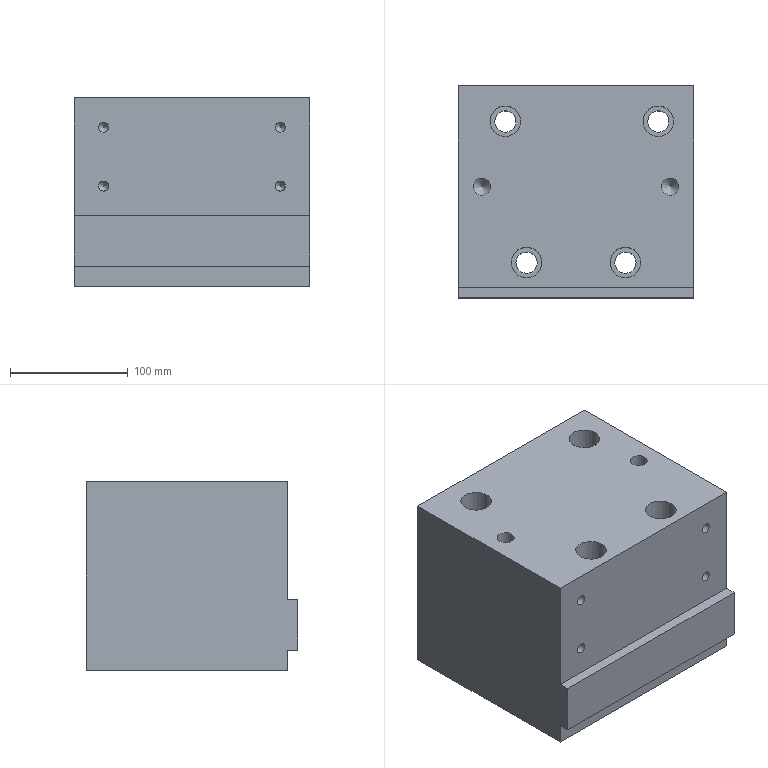Part | STEP file | lll_id3798_x_t | 1 solid | 34 faces | box 200 x 180 x 160 mm | volume 5233712 mm3 | plane 14 | cylinder 14 | cone 6 | commonest cylinder face diameters 8.506 x4 18.009 x4 26.008 x4 14.506 x2
STEP:
#1=CARTESIAN_POINT('',(1890.,537.377,65.));
#2=VERTEX_POINT('',#1);
#3=CARTESIAN_POINT('',(1890.,366.377,65.));
#4=VERTEX_POINT('',#3);
#5=CARTESIAN_POINT('',(1890.,293.877,65.));
#6=DIRECTION('',(0.,-1.,0.));
#7=VECTOR('',#6,1.);
#8=LINE('',#5,#7);
#9=EDGE_CURVE('',#2,#4,#8,.T.);
#10=ORIENTED_EDGE('',*,*,#9,.F.);
#11=CARTESIAN_POINT('',(1690.,537.377,65.));
#12=VERTEX_POINT('',#11);
#13=CARTESIAN_POINT('',(1665.,537.377,65.));
#14=DIRECTION('',(1.,0.,0.));
#15=VECTOR('',#14,1.);
#16=LINE('',#13,#15);
#17=EDGE_CURVE('',#12,#2,#16,.T.);
#18=ORIENTED_EDGE('',*,*,#17,.F.);
#19=CARTESIAN_POINT('',(1690.,366.377,65.));
#20=VERTEX_POINT('',#19);
#21=CARTESIAN_POINT('',(1690.,293.877,65.));
#22=DIRECTION('',(0.,1.,0.));
#23=VECTOR('',#22,1.);
#24=LINE('',#21,#23);
#25=EDGE_CURVE('',#20,#12,#24,.T.);
#26=ORIENTED_EDGE('',*,*,#25,.F.);
#27=CARTESIAN_POINT('',(1665.,366.377,65.));
#28=DIRECTION('',(-1.,0.,0.));
#29=VECTOR('',#28,1.);
#30=LINE('',#27,#29);
#31=EDGE_CURVE('',#4,#20,#30,.T.);
#32=ORIENTED_EDGE('',*,*,#31,.F.);
#33=EDGE_LOOP('',(#10,#18,#26,#32));
#34=FACE_BOUND('',#33,.T.);
#35=CARTESIAN_POINT('',(1873.004,507.377,65.));
#36=VERTEX_POINT('',#35);
#37=CARTESIAN_POINT('',(1860.,507.377,65.));
#38=DIRECTION('',(0.,0.,-1.));
#39=DIRECTION('',(1.,0.,0.));
#40=AXIS2_PLACEMENT_3D('',#37,#38,#39);
#41=CIRCLE('',#40,13.004);
#42=EDGE_CURVE('',#36,#36,#41,.T.);
#43=ORIENTED_EDGE('',*,*,#42,.T.);
#44=EDGE_LOOP('',(#43));
#45=FACE_BOUND('',#44,.T.);
#46=CARTESIAN_POINT('',(1845.004,387.377,65.));
#47=VERTEX_POINT('',#46);
#48=CARTESIAN_POINT('',(1832.,387.377,65.));
#49=DIRECTION('',(0.,0.,-1.));
#50=DIRECTION('',(1.,0.,0.));
#51=AXIS2_PLACEMENT_3D('',#48,#49,#50);
#52=CIRCLE('',#51,13.004);
#53=EDGE_CURVE('',#47,#47,#52,.T.);
#54=ORIENTED_EDGE('',*,*,#53,.T.);
#55=EDGE_LOOP('',(#54));
#56=FACE_BOUND('',#55,.T.);
#57=CARTESIAN_POINT('',(1877.253,451.877,65.));
#58=VERTEX_POINT('',#57);
#59=CARTESIAN_POINT('',(1870.,451.877,65.));
#60=DIRECTION('',(0.,0.,-1.));
#61=DIRECTION('',(1.,0.,0.));
#62=AXIS2_PLACEMENT_3D('',#59,#60,#61);
#63=CIRCLE('',#62,7.253);
#64=EDGE_CURVE('',#58,#58,#63,.T.);
#65=ORIENTED_EDGE('',*,*,#64,.T.);
#66=EDGE_LOOP('',(#65));
#67=FACE_BOUND('',#66,.T.);
#68=CARTESIAN_POINT('',(1702.747,451.877,65.));
#69=VERTEX_POINT('',#68);
#70=CARTESIAN_POINT('',(1710.,451.877,65.));
#71=DIRECTION('',(0.,0.,1.));
#72=DIRECTION('',(-1.,0.,0.));
#73=AXIS2_PLACEMENT_3D('',#70,#71,#72);
#74=CIRCLE('',#73,7.253);
#75=EDGE_CURVE('',#69,#69,#74,.T.);
#76=ORIENTED_EDGE('',*,*,#75,.F.);
#77=EDGE_LOOP('',(#76));
#78=FACE_BOUND('',#77,.T.);
#79=CARTESIAN_POINT('',(1734.996,387.377,65.));
#80=VERTEX_POINT('',#79);
#81=CARTESIAN_POINT('',(1748.,387.377,65.));
#82=DIRECTION('',(0.,0.,-1.));
#83=DIRECTION('',(-1.,0.,0.));
#84=AXIS2_PLACEMENT_3D('',#81,#82,#83);
#85=CIRCLE('',#84,13.004);
#86=EDGE_CURVE('',#80,#80,#85,.T.);
#87=ORIENTED_EDGE('',*,*,#86,.T.);
#88=EDGE_LOOP('',(#87));
#89=FACE_BOUND('',#88,.T.);
#90=CARTESIAN_POINT('',(1716.996,507.377,65.));
#91=VERTEX_POINT('',#90);
#92=CARTESIAN_POINT('',(1730.,507.377,65.));
#93=DIRECTION('',(0.,0.,-1.));
#94=DIRECTION('',(-1.,0.,0.));
#95=AXIS2_PLACEMENT_3D('',#92,#93,#94);
#96=CIRCLE('',#95,13.004);
#97=EDGE_CURVE('',#91,#91,#96,.T.);
#98=ORIENTED_EDGE('',*,*,#97,.T.);
#99=EDGE_LOOP('',(#98));
#100=FACE_BOUND('',#99,.T.);
#101=CARTESIAN_POINT('',(1665.,293.877,65.));
#102=DIRECTION('',(0.,0.,1.));
#103=DIRECTION('',(-1.,0.,0.));
#104=AXIS2_PLACEMENT_3D('',#101,#102,#103);
#105=PLANE('',#104);
#106=ADVANCED_FACE('',(#34,#45,#56,#67,#78,#89,#100),#105,.T.);
#107=CARTESIAN_POINT('',(1890.,537.377,-95.));
#108=VERTEX_POINT('',#107);
#109=CARTESIAN_POINT('',(1890.,537.377,-120.));
#110=DIRECTION('',(0.,0.,1.));
#111=VECTOR('',#110,1.);
#112=LINE('',#109,#111);
#113=EDGE_CURVE('',#108,#2,#112,.T.);
#114=ORIENTED_EDGE('',*,*,#113,.F.);
#115=CARTESIAN_POINT('',(1690.,537.377,-95.));
#116=VERTEX_POINT('',#115);
#117=CARTESIAN_POINT('',(1665.,537.377,-95.));
#118=DIRECTION('',(1.,0.,0.));
#119=VECTOR('',#118,1.);
#120=LINE('',#117,#119);
#121=EDGE_CURVE('',#116,#108,#120,.T.);
#122=ORIENTED_EDGE('',*,*,#121,.F.);
#123=CARTESIAN_POINT('',(1690.,537.377,-105.));
#124=DIRECTION('',(0.,0.,1.));
#125=VECTOR('',#124,1.);
#126=LINE('',#123,#125);
#127=EDGE_CURVE('',#116,#12,#126,.T.);
#128=ORIENTED_EDGE('',*,*,#127,.T.);
#129=ORIENTED_EDGE('',*,*,#17,.T.);
#130=EDGE_LOOP('',(#114,#122,#128,#129));
#131=FACE_OUTER_BOUND('',#130,.T.);
#132=CARTESIAN_POINT('',(1665.,537.377,-120.));
#133=DIRECTION('',(0.,1.,0.));
#134=DIRECTION('',(0.,0.,-1.));
#135=AXIS2_PLACEMENT_3D('',#132,#133,#134);
#136=PLANE('',#135);
#137=ADVANCED_FACE('',(#131),#136,.T.);
#138=CARTESIAN_POINT('',(1841.005,387.377,-55.));
#139=VERTEX_POINT('',#138);
#140=CARTESIAN_POINT('',(1832.,387.377,-55.));
#141=DIRECTION('',(0.,0.,-1.));
#142=DIRECTION('',(1.,0.,0.));
#143=AXIS2_PLACEMENT_3D('',#140,#141,#142);
#144=CIRCLE('',#143,9.005);
#145=EDGE_CURVE('',#139,#139,#144,.T.);
#146=ORIENTED_EDGE('',*,*,#145,.T.);
#147=EDGE_LOOP('',(#146));
#148=FACE_BOUND('',#147,.T.);
#149=CARTESIAN_POINT('',(1845.004,387.377,-55.));
#150=VERTEX_POINT('',#149);
#151=CARTESIAN_POINT('',(1832.,387.377,-55.));
#152=DIRECTION('',(0.,0.,-1.));
#153=DIRECTION('',(1.,0.,0.));
#154=AXIS2_PLACEMENT_3D('',#151,#152,#153);
#155=CIRCLE('',#154,13.004);
#156=EDGE_CURVE('',#150,#150,#155,.T.);
#157=ORIENTED_EDGE('',*,*,#156,.F.);
#158=EDGE_LOOP('',(#157));
#159=FACE_BOUND('',#158,.T.);
#160=CARTESIAN_POINT('',(1832.,387.377,-55.));
#161=DIRECTION('',(0.,0.,-1.));
#162=DIRECTION('',(-1.,0.,0.));
#163=AXIS2_PLACEMENT_3D('',#160,#161,#162);
#164=PLANE('',#163);
#165=ADVANCED_FACE('',(#148,#159),#164,.F.);
#166=ORIENTED_EDGE('',*,*,#145,.F.);
#167=EDGE_LOOP('',(#166));
#168=FACE_BOUND('',#167,.T.);
#169=CARTESIAN_POINT('',(1841.005,387.377,-95.));
#170=VERTEX_POINT('',#169);
#171=CARTESIAN_POINT('',(1832.,387.377,-95.));
#172=DIRECTION('',(0.,0.,-1.));
#173=DIRECTION('',(1.,0.,0.));
#174=AXIS2_PLACEMENT_3D('',#171,#172,#173);
#175=CIRCLE('',#174,9.005);
#176=EDGE_CURVE('',#170,#170,#175,.T.);
#177=ORIENTED_EDGE('',*,*,#176,.T.);
#178=EDGE_LOOP('',(#177));
#179=FACE_BOUND('',#178,.T.);
#180=CARTESIAN_POINT('',(1832.,387.377,67.));
#181=DIRECTION('',(0.,0.,-1.));
#182=DIRECTION('',(1.,0.,0.));
#183=AXIS2_PLACEMENT_3D('',#180,#181,#182);
#184=CYLINDRICAL_SURFACE('',#183,9.005);
#185=ADVANCED_FACE('',(#168,#179),#184,.F.);
#186=ORIENTED_EDGE('',*,*,#156,.T.);
#187=EDGE_LOOP('',(#186));
#188=FACE_BOUND('',#187,.T.);
#189=ORIENTED_EDGE('',*,*,#53,.F.);
#190=EDGE_LOOP('',(#189));
#191=FACE_BOUND('',#190,.T.);
#192=CARTESIAN_POINT('',(1832.,387.377,65.));
#193=DIRECTION('',(0.,0.,-1.));
#194=DIRECTION('',(1.,0.,0.));
#195=AXIS2_PLACEMENT_3D('',#192,#193,#194);
#196=CYLINDRICAL_SURFACE('',#195,13.004);
#197=ADVANCED_FACE('',(#188,#191),#196,.F.);
#198=CARTESIAN_POINT('',(1715.,401.383,40.));
#199=VERTEX_POINT('',#198);
#200=VERTEX_LOOP('',#199);
#201=FACE_BOUND('',#200,.T.);
#202=CARTESIAN_POINT('',(1715.,397.13,35.747));
#203=VERTEX_POINT('',#202);
#204=CARTESIAN_POINT('',(1715.,397.13,40.));
#205=DIRECTION('',(0.,1.,0.));
#206=DIRECTION('',(0.,0.,-1.));
#207=AXIS2_PLACEMENT_3D('',#204,#205,#206);
#208=CIRCLE('',#207,4.253);
#209=EDGE_CURVE('',#203,#203,#208,.T.);
#210=ORIENTED_EDGE('',*,*,#209,.F.);
#211=EDGE_LOOP('',(#210));
#212=FACE_BOUND('',#211,.T.);
#213=CARTESIAN_POINT('',(1715.,397.13,40.));
#214=DIRECTION('',(0.,-1.,0.));
#215=DIRECTION('',(0.,0.,1.));
#216=AXIS2_PLACEMENT_3D('',#213,#214,#215);
#217=CONICAL_SURFACE('',#216,4.253,45.);
#218=ADVANCED_FACE('',(#201,#212),#217,.F.);
#219=CARTESIAN_POINT('',(1865.,401.383,40.));
#220=VERTEX_POINT('',#219);
#221=VERTEX_LOOP('',#220);
#222=FACE_BOUND('',#221,.T.);
#223=CARTESIAN_POINT('',(1865.,397.13,35.747));
#224=VERTEX_POINT('',#223);
#225=CARTESIAN_POINT('',(1865.,397.13,40.));
#226=DIRECTION('',(0.,1.,0.));
#227=DIRECTION('',(0.,0.,-1.));
#228=AXIS2_PLACEMENT_3D('',#225,#226,#227);
#229=CIRCLE('',#228,4.253);
#230=EDGE_CURVE('',#224,#224,#229,.T.);
#231=ORIENTED_EDGE('',*,*,#230,.F.);
#232=EDGE_LOOP('',(#231));
#233=FACE_BOUND('',#232,.T.);
#234=CARTESIAN_POINT('',(1865.,397.13,40.));
#235=DIRECTION('',(0.,-1.,0.));
#236=DIRECTION('',(0.,0.,1.));
#237=AXIS2_PLACEMENT_3D('',#234,#235,#236);
#238=CONICAL_SURFACE('',#237,4.253,45.);
#239=ADVANCED_FACE('',(#222,#233),#238,.F.);
#240=CARTESIAN_POINT('',(1715.,401.383,-10.));
#241=VERTEX_POINT('',#240);
#242=VERTEX_LOOP('',#241);
#243=FACE_BOUND('',#242,.T.);
#244=CARTESIAN_POINT('',(1715.,397.13,-14.253));
#245=VERTEX_POINT('',#244);
#246=CARTESIAN_POINT('',(1715.,397.13,-10.));
#247=DIRECTION('',(0.,1.,0.));
#248=DIRECTION('',(0.,0.,-1.));
#249=AXIS2_PLACEMENT_3D('',#246,#247,#248);
#250=CIRCLE('',#249,4.253);
#251=EDGE_CURVE('',#245,#245,#250,.T.);
#252=ORIENTED_EDGE('',*,*,#251,.F.);
#253=EDGE_LOOP('',(#252));
#254=FACE_BOUND('',#253,.T.);
#255=CARTESIAN_POINT('',(1715.,397.13,-10.));
#256=DIRECTION('',(0.,-1.,0.));
#257=DIRECTION('',(0.,0.,1.));
#258=AXIS2_PLACEMENT_3D('',#255,#256,#257);
#259=CONICAL_SURFACE('',#258,4.253,45.);
#260=ADVANCED_FACE('',(#243,#254),#259,.F.);
#261=CARTESIAN_POINT('',(1865.,401.383,-10.));
#262=VERTEX_POINT('',#261);
#263=VERTEX_LOOP('',#262);
#264=FACE_BOUND('',#263,.T.);
#265=CARTESIAN_POINT('',(1865.,397.13,-14.253));
#266=VERTEX_POINT('',#265);
#267=CARTESIAN_POINT('',(1865.,397.13,-10.));
#268=DIRECTION('',(0.,1.,0.));
#269=DIRECTION('',(0.,0.,-1.));
#270=AXIS2_PLACEMENT_3D('',#267,#268,#269);
#271=CIRCLE('',#270,4.253);
#272=EDGE_CURVE('',#266,#266,#271,.T.);
#273=ORIENTED_EDGE('',*,*,#272,.F.);
#274=EDGE_LOOP('',(#273));
#275=FACE_BOUND('',#274,.T.);
#276=CARTESIAN_POINT('',(1865.,397.13,-10.));
#277=DIRECTION('',(0.,-1.,0.));
#278=DIRECTION('',(0.,0.,1.));
#279=AXIS2_PLACEMENT_3D('',#276,#277,#278);
#280=CONICAL_SURFACE('',#279,4.253,45.);
#281=ADVANCED_FACE('',(#264,#275),#280,.F.);
#282=CARTESIAN_POINT('',(1710.,451.877,21.994));
#283=VERTEX_POINT('',#282);
#284=VERTEX_LOOP('',#283);
#285=FACE_BOUND('',#284,.T.);
#286=CARTESIAN_POINT('',(1717.253,451.877,29.247));
#287=VERTEX_POINT('',#286);
#288=CARTESIAN_POINT('',(1710.,451.877,29.247));
#289=DIRECTION('',(0.,0.,-1.));
#290=DIRECTION('',(1.,0.,0.));
#291=AXIS2_PLACEMENT_3D('',#288,#289,#290);
#292=CIRCLE('',#291,7.253);
#293=EDGE_CURVE('',#287,#287,#292,.T.);
#294=ORIENTED_EDGE('',*,*,#293,.F.);
#295=EDGE_LOOP('',(#294));
#296=FACE_BOUND('',#295,.T.);
#297=CARTESIAN_POINT('',(1710.,451.877,29.247));
#298=DIRECTION('',(0.,0.,1.));
#299=DIRECTION('',(-1.,0.,0.));
#300=AXIS2_PLACEMENT_3D('',#297,#298,#299);
#301=CONICAL_SURFACE('',#300,7.253,45.);
#302=ADVANCED_FACE('',(#285,#296),#301,.F.);
#303=ORIENTED_EDGE('',*,*,#209,.T.);
#304=EDGE_LOOP('',(#303));
#305=FACE_BOUND('',#304,.T.);
#306=CARTESIAN_POINT('',(1710.747,366.377,40.));
#307=VERTEX_POINT('',#306);
#308=CARTESIAN_POINT('',(1715.,366.377,40.));
#309=DIRECTION('',(0.,1.,0.));
#310=DIRECTION('',(-1.,0.,0.));
#311=AXIS2_PLACEMENT_3D('',#308,#309,#310);
#312=CIRCLE('',#311,4.253);
#313=EDGE_CURVE('',#307,#307,#312,.T.);
#314=ORIENTED_EDGE('',*,*,#313,.F.);
#315=EDGE_LOOP('',(#314));
#316=FACE_BOUND('',#315,.T.);
#317=CARTESIAN_POINT('',(1715.,366.377,40.));
#318=DIRECTION('',(0.,1.,0.));
#319=DIRECTION('',(-1.,0.,0.));
#320=AXIS2_PLACEMENT_3D('',#317,#318,#319);
#321=CYLINDRICAL_SURFACE('',#320,4.253);
#322=ADVANCED_FACE('',(#305,#316),#321,.F.);
#323=ORIENTED_EDGE('',*,*,#230,.T.);
#324=EDGE_LOOP('',(#323));
#325=FACE_BOUND('',#324,.T.);
#326=CARTESIAN_POINT('',(1860.747,366.377,40.));
#327=VERTEX_POINT('',#326);
#328=CARTESIAN_POINT('',(1865.,366.377,40.));
#329=DIRECTION('',(0.,1.,0.));
#330=DIRECTION('',(-1.,0.,0.));
#331=AXIS2_PLACEMENT_3D('',#328,#329,#330);
#332=CIRCLE('',#331,4.253);
#333=EDGE_CURVE('',#327,#327,#332,.T.);
#334=ORIENTED_EDGE('',*,*,#333,.F.);
#335=EDGE_LOOP('',(#334));
#336=FACE_BOUND('',#335,.T.);
#337=CARTESIAN_POINT('',(1865.,366.377,40.));
#338=DIRECTION('',(0.,1.,0.));
#339=DIRECTION('',(-1.,0.,0.));
#340=AXIS2_PLACEMENT_3D('',#337,#338,#339);
#341=CYLINDRICAL_SURFACE('',#340,4.253);
#342=ADVANCED_FACE('',(#325,#336),#341,.F.);
#343=ORIENTED_EDGE('',*,*,#251,.T.);
#344=EDGE_LOOP('',(#343));
#345=FACE_BOUND('',#344,.T.);
#346=CARTESIAN_POINT('',(1710.747,366.377,-10.));
#347=VERTEX_POINT('',#346);
#348=CARTESIAN_POINT('',(1715.,366.377,-10.));
#349=DIRECTION('',(0.,1.,0.));
#350=DIRECTION('',(-1.,0.,0.));
#351=AXIS2_PLACEMENT_3D('',#348,#349,#350);
#352=CIRCLE('',#351,4.253);
#353=EDGE_CURVE('',#347,#347,#352,.T.);
#354=ORIENTED_EDGE('',*,*,#353,.F.);
#355=EDGE_LOOP('',(#354));
#356=FACE_BOUND('',#355,.T.);
#357=CARTESIAN_POINT('',(1715.,366.377,-10.));
#358=DIRECTION('',(0.,1.,0.));
#359=DIRECTION('',(-1.,0.,0.));
#360=AXIS2_PLACEMENT_3D('',#357,#358,#359);
#361=CYLINDRICAL_SURFACE('',#360,4.253);
#362=ADVANCED_FACE('',(#345,#356),#361,.F.);
#363=ORIENTED_EDGE('',*,*,#272,.T.);
#364=EDGE_LOOP('',(#363));
#365=FACE_BOUND('',#364,.T.);
#366=CARTESIAN_POINT('',(1860.747,366.377,-10.));
#367=VERTEX_POINT('',#366);
#368=CARTESIAN_POINT('',(1865.,366.377,-10.));
#369=DIRECTION('',(0.,1.,0.));
#370=DIRECTION('',(-1.,0.,0.));
#371=AXIS2_PLACEMENT_3D('',#368,#369,#370);
#372=CIRCLE('',#371,4.253);
#373=EDGE_CURVE('',#367,#367,#372,.T.);
#374=ORIENTED_EDGE('',*,*,#373,.F.);
#375=EDGE_LOOP('',(#374));
#376=FACE_BOUND('',#375,.T.);
#377=CARTESIAN_POINT('',(1865.,366.377,-10.));
#378=DIRECTION('',(0.,1.,0.));
#379=DIRECTION('',(-1.,0.,0.));
#380=AXIS2_PLACEMENT_3D('',#377,#378,#379);
#381=CYLINDRICAL_SURFACE('',#380,4.253);
#382=ADVANCED_FACE('',(#365,#376),#381,.F.);
#383=CARTESIAN_POINT('',(1738.995,387.377,-55.));
#384=VERTEX_POINT('',#383);
#385=CARTESIAN_POINT('',(1748.,387.377,-55.));
#386=DIRECTION('',(0.,0.,-1.));
#387=DIRECTION('',(-1.,0.,0.));
#388=AXIS2_PLACEMENT_3D('',#385,#386,#387);
#389=CIRCLE('',#388,9.005);
#390=EDGE_CURVE('',#384,#384,#389,.T.);
#391=ORIENTED_EDGE('',*,*,#390,.T.);
#392=EDGE_LOOP('',(#391));
#393=FACE_BOUND('',#392,.T.);
#394=CARTESIAN_POINT('',(1734.996,387.377,-55.));
#395=VERTEX_POINT('',#394);
#396=CARTESIAN_POINT('',(1748.,387.377,-55.));
#397=DIRECTION('',(0.,0.,-1.));
#398=DIRECTION('',(-1.,0.,0.));
#399=AXIS2_PLACEMENT_3D('',#396,#397,#398);
#400=CIRCLE('',#399,13.004);
#401=EDGE_CURVE('',#395,#395,#400,.T.);
#402=ORIENTED_EDGE('',*,*,#401,.F.);
#403=EDGE_LOOP('',(#402));
#404=FACE_BOUND('',#403,.T.);
#405=CARTESIAN_POINT('',(1748.,387.377,-55.));
#406=DIRECTION('',(0.,0.,-1.));
#407=DIRECTION('',(1.,0.,0.));
#408=AXIS2_PLACEMENT_3D('',#405,#406,#407);
#409=PLANE('',#408);
#410=ADVANCED_FACE('',(#393,#404),#409,.F.);
#411=CARTESIAN_POINT('',(1690.,366.377,-35.));
#412=VERTEX_POINT('',#411);
#413=CARTESIAN_POINT('',(1890.,366.377,-35.));
#414=VERTEX_POINT('',#413);
#415=CARTESIAN_POINT('',(1142.435,366.377,-35.));
#416=DIRECTION('',(1.,0.,0.));
#417=VECTOR('',#416,1.);
#418=LINE('',#415,#417);
#419=EDGE_CURVE('',#412,#414,#418,.T.);
#420=ORIENTED_EDGE('',*,*,#419,.F.);
#421=CARTESIAN_POINT('',(1690.,357.377,-35.));
#422=VERTEX_POINT('',#421);
#423=CARTESIAN_POINT('',(1690.,376.377,-35.));
#424=DIRECTION('',(0.,1.,0.));
#425=VECTOR('',#424,1.);
#426=LINE('',#423,#425);
#427=EDGE_CURVE('',#422,#412,#426,.T.);
#428=ORIENTED_EDGE('',*,*,#427,.F.);
#429=CARTESIAN_POINT('',(1890.,357.377,-35.));
#430=VERTEX_POINT('',#429);
#431=CARTESIAN_POINT('',(1142.435,357.377,-35.));
#432=DIRECTION('',(-1.,0.,0.));
#433=VECTOR('',#432,1.);
#434=LINE('',#431,#433);
#435=EDGE_CURVE('',#430,#422,#434,.T.);
#436=ORIENTED_EDGE('',*,*,#435,.F.);
#437=CARTESIAN_POINT('',(1890.,26.33,-35.));
#438=DIRECTION('',(0.,1.,0.));
#439=VECTOR('',#438,1.);
#440=LINE('',#437,#439);
#441=EDGE_CURVE('',#430,#414,#440,.T.);
#442=ORIENTED_EDGE('',*,*,#441,.T.);
#443=EDGE_LOOP('',(#420,#428,#436,#442));
#444=FACE_OUTER_BOUND('',#443,.T.);
#445=CARTESIAN_POINT('',(1142.435,26.33,-35.));
#446=DIRECTION('',(0.,0.,1.));
#447=DIRECTION('',(1.,0.,0.));
#448=AXIS2_PLACEMENT_3D('',#445,#446,#447);
#449=PLANE('',#448);
#450=ADVANCED_FACE('',(#444),#449,.T.);
#451=CARTESIAN_POINT('',(1720.995,507.377,-55.));
#452=VERTEX_POINT('',#451);
#453=CARTESIAN_POINT('',(1730.,507.377,-55.));
#454=DIRECTION('',(0.,0.,-1.));
#455=DIRECTION('',(-1.,0.,0.));
#456=AXIS2_PLACEMENT_3D('',#453,#454,#455);
#457=CIRCLE('',#456,9.005);
#458=EDGE_CURVE('',#452,#452,#457,.T.);
#459=ORIENTED_EDGE('',*,*,#458,.T.);
#460=EDGE_LOOP('',(#459));
#461=FACE_BOUND('',#460,.T.);
#462=CARTESIAN_POINT('',(1716.996,507.377,-55.));
#463=VERTEX_POINT('',#462);
#464=CARTESIAN_POINT('',(1730.,507.377,-55.));
#465=DIRECTION('',(0.,0.,-1.));
#466=DIRECTION('',(-1.,0.,0.));
#467=AXIS2_PLACEMENT_3D('',#464,#465,#466);
#468=CIRCLE('',#467,13.004);
#469=EDGE_CURVE('',#463,#463,#468,.T.);
#470=ORIENTED_EDGE('',*,*,#469,.F.);
#471=EDGE_LOOP('',(#470));
#472=FACE_BOUND('',#471,.T.);
#473=CARTESIAN_POINT('',(1730.,507.377,-55.));
#474=DIRECTION('',(0.,0.,-1.));
#475=DIRECTION('',(1.,0.,0.));
#476=AXIS2_PLACEMENT_3D('',#473,#474,#475);
#477=PLANE('',#476);
#478=ADVANCED_FACE('',(#461,#472),#477,.F.);
#479=ORIENTED_EDGE('',*,*,#469,.T.);
#480=EDGE_LOOP('',(#479));
#481=FACE_BOUND('',#480,.T.);
#482=ORIENTED_EDGE('',*,*,#97,.F.);
#483=EDGE_LOOP('',(#482));
#484=FACE_BOUND('',#483,.T.);
#485=CARTESIAN_POINT('',(1730.,507.377,65.));
#486=DIRECTION('',(0.,0.,-1.));
#487=DIRECTION('',(-1.,0.,0.));
#488=AXIS2_PLACEMENT_3D('',#485,#486,#487);
#489=CYLINDRICAL_SURFACE('',#488,13.004);
#490=ADVANCED_FACE('',(#481,#484),#489,.F.);
#491=ORIENTED_EDGE('',*,*,#401,.T.);
#492=EDGE_LOOP('',(#491));
#493=FACE_BOUND('',#492,.T.);
#494=ORIENTED_EDGE('',*,*,#86,.F.);
#495=EDGE_LOOP('',(#494));
#496=FACE_BOUND('',#495,.T.);
#497=CARTESIAN_POINT('',(1748.,387.377,65.));
#498=DIRECTION('',(0.,0.,-1.));
#499=DIRECTION('',(-1.,0.,0.));
#500=AXIS2_PLACEMENT_3D('',#497,#498,#499);
#501=CYLINDRICAL_SURFACE('',#500,13.004);
#502=ADVANCED_FACE('',(#493,#496),#501,.F.);
#503=ORIENTED_EDGE('',*,*,#75,.T.);
#504=EDGE_LOOP('',(#503));
#505=FACE_BOUND('',#504,.T.);
#506=ORIENTED_EDGE('',*,*,#293,.T.);
#507=EDGE_LOOP('',(#506));
#508=FACE_BOUND('',#507,.T.);
#509=CARTESIAN_POINT('',(1710.,451.877,67.));
#510=DIRECTION('',(0.,0.,-1.));
#511=DIRECTION('',(-1.,0.,0.));
#512=AXIS2_PLACEMENT_3D('',#509,#510,#511);
#513=CYLINDRICAL_SURFACE('',#512,7.253);
#514=ADVANCED_FACE('',(#505,#508),#513,.F.);
#515=ORIENTED_EDGE('',*,*,#373,.T.);
#516=EDGE_LOOP('',(#515));
#517=FACE_BOUND('',#516,.T.);
#518=ORIENTED_EDGE('',*,*,#353,.T.);
#519=EDGE_LOOP('',(#518));
#520=FACE_BOUND('',#519,.T.);
#521=ORIENTED_EDGE('',*,*,#333,.T.);
#522=EDGE_LOOP('',(#521));
#523=FACE_BOUND('',#522,.T.);
#524=ORIENTED_EDGE('',*,*,#313,.T.);
#525=EDGE_LOOP('',(#524));
#526=FACE_BOUND('',#525,.T.);
#527=ORIENTED_EDGE('',*,*,#31,.T.);
#528=CARTESIAN_POINT('',(1690.,366.377,130.851));
#529=DIRECTION('',(0.,0.,-1.));
#530=VECTOR('',#529,1.);
#531=LINE('',#528,#530);
#532=EDGE_CURVE('',#20,#412,#531,.T.);
#533=ORIENTED_EDGE('',*,*,#532,.T.);
#534=ORIENTED_EDGE('',*,*,#419,.T.);
#535=CARTESIAN_POINT('',(1890.,366.377,130.851));
#536=DIRECTION('',(0.,0.,-1.));
#537=VECTOR('',#536,1.);
#538=LINE('',#535,#537);
#539=EDGE_CURVE('',#4,#414,#538,.T.);
#540=ORIENTED_EDGE('',*,*,#539,.F.);
#541=EDGE_LOOP('',(#527,#533,#534,#540));
#542=FACE_BOUND('',#541,.T.);
#543=CARTESIAN_POINT('',(1695.,366.377,130.851));
#544=DIRECTION('',(0.,1.,0.));
#545=DIRECTION('',(0.,0.,-1.));
#546=AXIS2_PLACEMENT_3D('',#543,#544,#545);
#547=PLANE('',#546);
#548=ADVANCED_FACE('',(#517,#520,#523,#526,#542),#547,.F.);
#549=ORIENTED_EDGE('',*,*,#390,.F.);
#550=EDGE_LOOP('',(#549));
#551=FACE_BOUND('',#550,.T.);
#552=CARTESIAN_POINT('',(1757.005,387.377,-95.));
#553=VERTEX_POINT('',#552);
#554=CARTESIAN_POINT('',(1748.,387.377,-95.));
#555=DIRECTION('',(0.,0.,1.));
#556=DIRECTION('',(1.,0.,0.));
#557=AXIS2_PLACEMENT_3D('',#554,#555,#556);
#558=CIRCLE('',#557,9.005);
#559=EDGE_CURVE('',#553,#553,#558,.T.);
#560=ORIENTED_EDGE('',*,*,#559,.F.);
#561=EDGE_LOOP('',(#560));
#562=FACE_BOUND('',#561,.T.);
#563=CARTESIAN_POINT('',(1748.,387.377,67.));
#564=DIRECTION('',(0.,0.,-1.));
#565=DIRECTION('',(-1.,0.,0.));
#566=AXIS2_PLACEMENT_3D('',#563,#564,#565);
#567=CYLINDRICAL_SURFACE('',#566,9.005);
#568=ADVANCED_FACE('',(#551,#562),#567,.F.);
#569=CARTESIAN_POINT('',(1890.,357.377,-78.));
#570=VERTEX_POINT('',#569);
#571=CARTESIAN_POINT('',(1890.,357.377,-690.));
#572=DIRECTION('',(0.,0.,1.));
#573=VECTOR('',#572,1.);
#574=LINE('',#571,#573);
#575=EDGE_CURVE('',#570,#430,#574,.T.);
#576=ORIENTED_EDGE('',*,*,#575,.F.);
#577=CARTESIAN_POINT('',(1890.,366.377,-78.));
#578=VERTEX_POINT('',#577);
#579=CARTESIAN_POINT('',(1890.,416.877,-78.));
#580=DIRECTION('',(0.,1.,0.));
#581=VECTOR('',#580,1.);
#582=LINE('',#579,#581);
#583=EDGE_CURVE('',#570,#578,#582,.T.);
#584=ORIENTED_EDGE('',*,*,#583,.T.);
#585=CARTESIAN_POINT('',(1890.,366.377,-95.));
#586=VERTEX_POINT('',#585);
#587=CARTESIAN_POINT('',(1890.,366.377,-35.));
#588=DIRECTION('',(0.,0.,1.));
#589=VECTOR('',#588,1.);
#590=LINE('',#587,#589);
#591=EDGE_CURVE('',#586,#578,#590,.T.);
#592=ORIENTED_EDGE('',*,*,#591,.F.);
#593=CARTESIAN_POINT('',(1890.,416.877,-95.));
#594=DIRECTION('',(0.,1.,0.));
#595=VECTOR('',#594,1.);
#596=LINE('',#593,#595);
#597=EDGE_CURVE('',#586,#108,#596,.T.);
#598=ORIENTED_EDGE('',*,*,#597,.T.);
#599=ORIENTED_EDGE('',*,*,#113,.T.);
#600=ORIENTED_EDGE('',*,*,#9,.T.);
#601=ORIENTED_EDGE('',*,*,#539,.T.);
#602=ORIENTED_EDGE('',*,*,#441,.F.);
#603=EDGE_LOOP('',(#576,#584,#592,#598,#599,#600,#601,#602));
#604=FACE_OUTER_BOUND('',#603,.T.);
#605=CARTESIAN_POINT('',(1890.,416.877,-35.));
#606=DIRECTION('',(-1.,0.,0.));
#607=DIRECTION('',(0.,0.,1.));
#608=AXIS2_PLACEMENT_3D('',#605,#606,#607);
#609=PLANE('',#608);
#610=ADVANCED_FACE('',(#604),#609,.F.);
#611=CARTESIAN_POINT('',(1690.,357.377,-78.));
#612=VERTEX_POINT('',#611);
#613=CARTESIAN_POINT('',(-3186.249,357.377,-78.));
#614=DIRECTION('',(-1.,0.,0.));
#615=VECTOR('',#614,1.);
#616=LINE('',#613,#615);
#617=EDGE_CURVE('',#570,#612,#616,.T.);
#618=ORIENTED_EDGE('',*,*,#617,.F.);
#619=ORIENTED_EDGE('',*,*,#575,.T.);
#620=ORIENTED_EDGE('',*,*,#435,.T.);
#621=CARTESIAN_POINT('',(1690.,357.377,-105.));
#622=DIRECTION('',(0.,0.,-1.));
#623=VECTOR('',#622,1.);
#624=LINE('',#621,#623);
#625=EDGE_CURVE('',#422,#612,#624,.T.);
#626=ORIENTED_EDGE('',*,*,#625,.T.);
#627=EDGE_LOOP('',(#618,#619,#620,#626));
#628=FACE_OUTER_BOUND('',#627,.T.);
#629=CARTESIAN_POINT('',(-3186.249,357.377,-690.));
#630=DIRECTION('',(0.,-1.,0.));
#631=DIRECTION('',(0.,0.,1.));
#632=AXIS2_PLACEMENT_3D('',#629,#630,#631);
#633=PLANE('',#632);
#634=ADVANCED_FACE('',(#628),#633,.T.);
#635=ORIENTED_EDGE('',*,*,#127,.F.);
#636=CARTESIAN_POINT('',(1690.,366.377,-95.));
#637=VERTEX_POINT('',#636);
#638=CARTESIAN_POINT('',(1690.,376.377,-95.));
#639=DIRECTION('',(0.,1.,0.));
#640=VECTOR('',#639,1.);
#641=LINE('',#638,#640);
#642=EDGE_CURVE('',#637,#116,#641,.T.);
#643=ORIENTED_EDGE('',*,*,#642,.F.);
#644=CARTESIAN_POINT('',(1690.,366.377,-78.));
#645=VERTEX_POINT('',#644);
#646=CARTESIAN_POINT('',(1690.,366.377,-105.));
#647=DIRECTION('',(0.,0.,-1.));
#648=VECTOR('',#647,1.);
#649=LINE('',#646,#648);
#650=EDGE_CURVE('',#645,#637,#649,.T.);
#651=ORIENTED_EDGE('',*,*,#650,.F.);
#652=CARTESIAN_POINT('',(1690.,0.000000688,-78.));
#653=DIRECTION('',(0.,1.,0.));
#654=VECTOR('',#653,1.);
#655=LINE('',#652,#654);
#656=EDGE_CURVE('',#612,#645,#655,.T.);
#657=ORIENTED_EDGE('',*,*,#656,.F.);
#658=ORIENTED_EDGE('',*,*,#625,.F.);
#659=ORIENTED_EDGE('',*,*,#427,.T.);
#660=ORIENTED_EDGE('',*,*,#532,.F.);
#661=ORIENTED_EDGE('',*,*,#25,.T.);
#662=EDGE_LOOP('',(#635,#643,#651,#657,#658,#659,#660,#661));
#663=FACE_OUTER_BOUND('',#662,.T.);
#664=CARTESIAN_POINT('',(1690.,376.377,-105.));
#665=DIRECTION('',(1.,0.,0.));
#666=DIRECTION('',(0.,0.,1.));
#667=AXIS2_PLACEMENT_3D('',#664,#665,#666);
#668=PLANE('',#667);
#669=ADVANCED_FACE('',(#663),#668,.F.);
#670=ORIENTED_EDGE('',*,*,#458,.F.);
#671=EDGE_LOOP('',(#670));
#672=FACE_BOUND('',#671,.T.);
#673=CARTESIAN_POINT('',(1739.005,507.377,-95.));
#674=VERTEX_POINT('',#673);
#675=CARTESIAN_POINT('',(1730.,507.377,-95.));
#676=DIRECTION('',(0.,0.,1.));
#677=DIRECTION('',(1.,0.,0.));
#678=AXIS2_PLACEMENT_3D('',#675,#676,#677);
#679=CIRCLE('',#678,9.005);
#680=EDGE_CURVE('',#674,#674,#679,.T.);
#681=ORIENTED_EDGE('',*,*,#680,.F.);
#682=EDGE_LOOP('',(#681));
#683=FACE_BOUND('',#682,.T.);
#684=CARTESIAN_POINT('',(1730.,507.377,67.));
#685=DIRECTION('',(0.,0.,-1.));
#686=DIRECTION('',(-1.,0.,0.));
#687=AXIS2_PLACEMENT_3D('',#684,#685,#686);
#688=CYLINDRICAL_SURFACE('',#687,9.005);
#689=ADVANCED_FACE('',(#672,#683),#688,.F.);
#690=CARTESIAN_POINT('',(1869.005,507.377,-55.));
#691=VERTEX_POINT('',#690);
#692=CARTESIAN_POINT('',(1860.,507.377,-55.));
#693=DIRECTION('',(0.,0.,-1.));
#694=DIRECTION('',(1.,0.,0.));
#695=AXIS2_PLACEMENT_3D('',#692,#693,#694);
#696=CIRCLE('',#695,9.005);
#697=EDGE_CURVE('',#691,#691,#696,.T.);
#698=ORIENTED_EDGE('',*,*,#697,.T.);
#699=EDGE_LOOP('',(#698));
#700=FACE_BOUND('',#699,.T.);
#701=CARTESIAN_POINT('',(1873.004,507.377,-55.));
#702=VERTEX_POINT('',#701);
#703=CARTESIAN_POINT('',(1860.,507.377,-55.));
#704=DIRECTION('',(0.,0.,-1.));
#705=DIRECTION('',(1.,0.,0.));
#706=AXIS2_PLACEMENT_3D('',#703,#704,#705);
#707=CIRCLE('',#706,13.004);
#708=EDGE_CURVE('',#702,#702,#707,.T.);
#709=ORIENTED_EDGE('',*,*,#708,.F.);
#710=EDGE_LOOP('',(#709));
#711=FACE_BOUND('',#710,.T.);
#712=CARTESIAN_POINT('',(1860.,507.377,-55.));
#713=DIRECTION('',(0.,0.,-1.));
#714=DIRECTION('',(-1.,0.,0.));
#715=AXIS2_PLACEMENT_3D('',#712,#713,#714);
#716=PLANE('',#715);
#717=ADVANCED_FACE('',(#700,#711),#716,.F.);
#718=ORIENTED_EDGE('',*,*,#697,.F.);
#719=EDGE_LOOP('',(#718));
#720=FACE_BOUND('',#719,.T.);
#721=CARTESIAN_POINT('',(1869.005,507.377,-95.));
#722=VERTEX_POINT('',#721);
#723=CARTESIAN_POINT('',(1860.,507.377,-95.));
#724=DIRECTION('',(0.,0.,-1.));
#725=DIRECTION('',(1.,0.,0.));
#726=AXIS2_PLACEMENT_3D('',#723,#724,#725);
#727=CIRCLE('',#726,9.005);
#728=EDGE_CURVE('',#722,#722,#727,.T.);
#729=ORIENTED_EDGE('',*,*,#728,.T.);
#730=EDGE_LOOP('',(#729));
#731=FACE_BOUND('',#730,.T.);
#732=CARTESIAN_POINT('',(1860.,507.377,67.));
#733=DIRECTION('',(0.,0.,-1.));
#734=DIRECTION('',(1.,0.,0.));
#735=AXIS2_PLACEMENT_3D('',#732,#733,#734);
#736=CYLINDRICAL_SURFACE('',#735,9.005);
#737=ADVANCED_FACE('',(#720,#731),#736,.F.);
#738=ORIENTED_EDGE('',*,*,#708,.T.);
#739=EDGE_LOOP('',(#738));
#740=FACE_BOUND('',#739,.T.);
#741=ORIENTED_EDGE('',*,*,#42,.F.);
#742=EDGE_LOOP('',(#741));
#743=FACE_BOUND('',#742,.T.);
#744=CARTESIAN_POINT('',(1860.,507.377,65.));
#745=DIRECTION('',(0.,0.,-1.));
#746=DIRECTION('',(1.,0.,0.));
#747=AXIS2_PLACEMENT_3D('',#744,#745,#746);
#748=CYLINDRICAL_SURFACE('',#747,13.004);
#749=ADVANCED_FACE('',(#740,#743),#748,.F.);
#750=CARTESIAN_POINT('',(1870.,451.877,21.994));
#751=VERTEX_POINT('',#750);
#752=VERTEX_LOOP('',#751);
#753=FACE_BOUND('',#752,.T.);
#754=CARTESIAN_POINT('',(1862.747,451.877,29.247));
#755=VERTEX_POINT('',#754);
#756=CARTESIAN_POINT('',(1870.,451.877,29.247));
#757=DIRECTION('',(0.,0.,-1.));
#758=DIRECTION('',(-1.,0.,0.));
#759=AXIS2_PLACEMENT_3D('',#756,#757,#758);
#760=CIRCLE('',#759,7.253);
#761=EDGE_CURVE('',#755,#755,#760,.T.);
#762=ORIENTED_EDGE('',*,*,#761,.F.);
#763=EDGE_LOOP('',(#762));
#764=FACE_BOUND('',#763,.T.);
#765=CARTESIAN_POINT('',(1870.,451.877,29.247));
#766=DIRECTION('',(0.,0.,1.));
#767=DIRECTION('',(1.,0.,0.));
#768=AXIS2_PLACEMENT_3D('',#765,#766,#767);
#769=CONICAL_SURFACE('',#768,7.253,45.);
#770=ADVANCED_FACE('',(#753,#764),#769,.F.);
#771=ORIENTED_EDGE('',*,*,#64,.F.);
#772=EDGE_LOOP('',(#771));
#773=FACE_BOUND('',#772,.T.);
#774=ORIENTED_EDGE('',*,*,#761,.T.);
#775=EDGE_LOOP('',(#774));
#776=FACE_BOUND('',#775,.T.);
#777=CARTESIAN_POINT('',(1870.,451.877,67.));
#778=DIRECTION('',(0.,0.,-1.));
#779=DIRECTION('',(1.,0.,0.));
#780=AXIS2_PLACEMENT_3D('',#777,#778,#779);
#781=CYLINDRICAL_SURFACE('',#780,7.253);
#782=ADVANCED_FACE('',(#773,#776),#781,.F.);
#783=ORIENTED_EDGE('',*,*,#656,.T.);
#784=CARTESIAN_POINT('',(2067.435,366.377,-78.));
#785=DIRECTION('',(1.,0.,0.));
#786=VECTOR('',#785,1.);
#787=LINE('',#784,#786);
#788=EDGE_CURVE('',#645,#578,#787,.T.);
#789=ORIENTED_EDGE('',*,*,#788,.T.);
#790=ORIENTED_EDGE('',*,*,#583,.F.);
#791=ORIENTED_EDGE('',*,*,#617,.T.);
#792=EDGE_LOOP('',(#783,#789,#790,#791));
#793=FACE_OUTER_BOUND('',#792,.T.);
#794=CARTESIAN_POINT('',(2067.435,0.000000688,-78.));
#795=DIRECTION('',(0.,0.,1.));
#796=DIRECTION('',(-1.,0.,0.));
#797=AXIS2_PLACEMENT_3D('',#794,#795,#796);
#798=PLANE('',#797);
#799=ADVANCED_FACE('',(#793),#798,.F.);
#800=ORIENTED_EDGE('',*,*,#591,.T.);
#801=ORIENTED_EDGE('',*,*,#788,.F.);
#802=ORIENTED_EDGE('',*,*,#650,.T.);
#803=CARTESIAN_POINT('',(2092.435,366.377,-95.));
#804=DIRECTION('',(1.,0.,0.));
#805=VECTOR('',#804,1.);
#806=LINE('',#803,#805);
#807=EDGE_CURVE('',#637,#586,#806,.T.);
#808=ORIENTED_EDGE('',*,*,#807,.T.);
#809=EDGE_LOOP('',(#800,#801,#802,#808));
#810=FACE_OUTER_BOUND('',#809,.T.);
#811=CARTESIAN_POINT('',(1695.,366.377,130.851));
#812=DIRECTION('',(0.,1.,0.));
#813=DIRECTION('',(0.,0.,-1.));
#814=AXIS2_PLACEMENT_3D('',#811,#812,#813);
#815=PLANE('',#814);
#816=ADVANCED_FACE('',(#810),#815,.F.);
#817=ORIENTED_EDGE('',*,*,#642,.T.);
#818=ORIENTED_EDGE('',*,*,#121,.T.);
#819=ORIENTED_EDGE('',*,*,#597,.F.);
#820=ORIENTED_EDGE('',*,*,#807,.F.);
#821=EDGE_LOOP('',(#817,#818,#819,#820));
#822=FACE_BOUND('',#821,.T.);
#823=ORIENTED_EDGE('',*,*,#559,.T.);
#824=EDGE_LOOP('',(#823));
#825=FACE_BOUND('',#824,.T.);
#826=ORIENTED_EDGE('',*,*,#680,.T.);
#827=EDGE_LOOP('',(#826));
#828=FACE_BOUND('',#827,.T.);
#829=ORIENTED_EDGE('',*,*,#176,.F.);
#830=EDGE_LOOP('',(#829));
#831=FACE_BOUND('',#830,.T.);
#832=ORIENTED_EDGE('',*,*,#728,.F.);
#833=EDGE_LOOP('',(#832));
#834=FACE_BOUND('',#833,.T.);
#835=CARTESIAN_POINT('',(2092.435,-0.000000688,-95.));
#836=DIRECTION('',(0.,0.,1.));
#837=DIRECTION('',(1.,0.,0.));
#838=AXIS2_PLACEMENT_3D('',#835,#836,#837);
#839=PLANE('',#838);
#840=ADVANCED_FACE('',(#822,#825,#828,#831,#834),#839,.F.);
#841=CLOSED_SHELL('',(#106,#137,#165,#185,#197,#218,#239,#260,#281,#302,#322,#342,#362,#382,#410,#450,#478,#490,#502,#514,#548,#568,#610,#634,#669,#689,#717,#737,#749,#770,#782,#799,#816,#840));
#842=MANIFOLD_SOLID_BREP('',#841);
#843=(LENGTH_UNIT()NAMED_UNIT(*)SI_UNIT(.MILLI.,.METRE.));
#844=UNCERTAINTY_MEASURE_WITH_UNIT(LENGTH_MEASURE(0.00002),#843,'','');
#845=(NAMED_UNIT(*)PLANE_ANGLE_UNIT()SI_UNIT($,.RADIAN.));
#846=PLANE_ANGLE_MEASURE_WITH_UNIT(PLANE_ANGLE_MEASURE(0.01745),#845);
#847=DIMENSIONAL_EXPONENTS(0.,0.,0.,0.,0.,0.,0.);
#848=(CONVERSION_BASED_UNIT('DEGREE',#846)NAMED_UNIT(#847)PLANE_ANGLE_UNIT());
#849=(NAMED_UNIT(*)SI_UNIT($,.STERADIAN.)SOLID_ANGLE_UNIT());
#850=(GEOMETRIC_REPRESENTATION_CONTEXT(3)GLOBAL_UNCERTAINTY_ASSIGNED_CONTEXT((#844))GLOBAL_UNIT_ASSIGNED_CONTEXT((#843,#848,#849))REPRESENTATION_CONTEXT('',''));
#851=ADVANCED_BREP_SHAPE_REPRESENTATION('',(#842),#850);